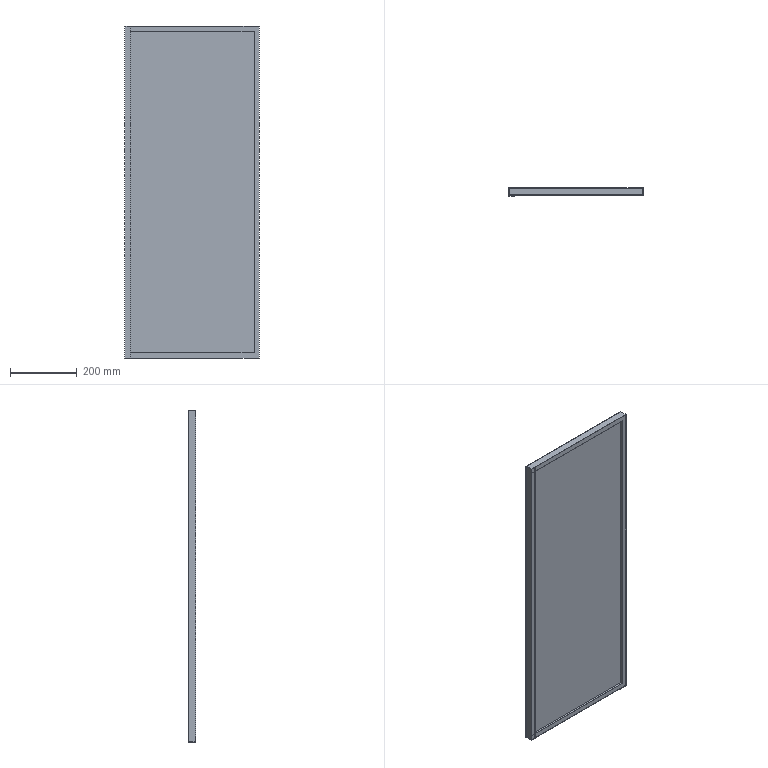Part | SolidWorks | features BossThin 2, ExtruThin 1 | 2 solids | 22 faces | box 401 x 23 x 992 mm | volume 497496 mm3 | plane 22
STEP:
#1=CARTESIAN_POINT('',(185.,-22.96,480.));
#2=VERTEX_POINT('',#1);
#3=CARTESIAN_POINT('',(-200.,-22.96,480.));
#4=VERTEX_POINT('',#3);
#5=CARTESIAN_POINT('',(200.,-22.96,480.));
#6=DIRECTION('',(-1.,0.,0.));
#7=VECTOR('',#6,1000.);
#8=LINE('',#5,#7);
#9=EDGE_CURVE('',#2,#4,#8,.T.);
#10=ORIENTED_EDGE('',*,*,#9,.F.);
#11=CARTESIAN_POINT('',(185.,-23.96,480.));
#12=VERTEX_POINT('',#11);
#13=CARTESIAN_POINT('',(185.,-22.96,480.));
#14=DIRECTION('',(0.,-1.,0.));
#15=VECTOR('',#14,1000.);
#16=LINE('',#13,#15);
#17=EDGE_CURVE('',#2,#12,#16,.T.);
#18=ORIENTED_EDGE('',*,*,#17,.T.);
#19=CARTESIAN_POINT('',(-200.,-23.96,480.));
#20=VERTEX_POINT('',#19);
#21=CARTESIAN_POINT('',(200.,-23.96,480.));
#22=DIRECTION('',(-1.,0.,0.));
#23=VECTOR('',#22,1000.);
#24=LINE('',#21,#23);
#25=EDGE_CURVE('',#12,#20,#24,.T.);
#26=ORIENTED_EDGE('',*,*,#25,.T.);
#27=CARTESIAN_POINT('',(-200.,-22.96,480.));
#28=DIRECTION('',(0.,-1.,0.));
#29=VECTOR('',#28,1000.);
#30=LINE('',#27,#29);
#31=EDGE_CURVE('',#4,#20,#30,.T.);
#32=ORIENTED_EDGE('',*,*,#31,.F.);
#33=EDGE_LOOP('',(#10,#18,#26,#32));
#34=FACE_OUTER_BOUND('',#33,.T.);
#35=CARTESIAN_POINT('',(200.,-22.96,480.));
#36=DIRECTION('',(0.,0.,-1.));
#37=DIRECTION('',(-1.,0.,0.));
#38=AXIS2_PLACEMENT_3D('',#35,#36,#37);
#39=PLANE('',#38);
#40=ADVANCED_FACE('',(#34),#39,.T.);
#41=CARTESIAN_POINT('',(185.,-23.96,-480.));
#42=VERTEX_POINT('',#41);
#43=CARTESIAN_POINT('',(-200.,-23.96,-480.));
#44=VERTEX_POINT('',#43);
#45=CARTESIAN_POINT('',(200.,-23.96,-480.));
#46=DIRECTION('',(-1.,0.,0.));
#47=VECTOR('',#46,1000.);
#48=LINE('',#45,#47);
#49=EDGE_CURVE('',#42,#44,#48,.T.);
#50=ORIENTED_EDGE('',*,*,#49,.F.);
#51=CARTESIAN_POINT('',(185.,-22.96,-480.));
#52=VERTEX_POINT('',#51);
#53=CARTESIAN_POINT('',(185.,-23.96,-480.));
#54=DIRECTION('',(0.,1.,0.));
#55=VECTOR('',#54,1000.);
#56=LINE('',#53,#55);
#57=EDGE_CURVE('',#42,#52,#56,.T.);
#58=ORIENTED_EDGE('',*,*,#57,.T.);
#59=CARTESIAN_POINT('',(-200.,-22.96,-480.));
#60=VERTEX_POINT('',#59);
#61=CARTESIAN_POINT('',(200.,-22.96,-480.));
#62=DIRECTION('',(-1.,0.,0.));
#63=VECTOR('',#62,1000.);
#64=LINE('',#61,#63);
#65=EDGE_CURVE('',#52,#60,#64,.T.);
#66=ORIENTED_EDGE('',*,*,#65,.T.);
#67=CARTESIAN_POINT('',(-200.,-23.96,-480.));
#68=DIRECTION('',(0.,1.,0.));
#69=VECTOR('',#68,1000.);
#70=LINE('',#67,#69);
#71=EDGE_CURVE('',#44,#60,#70,.T.);
#72=ORIENTED_EDGE('',*,*,#71,.F.);
#73=EDGE_LOOP('',(#50,#58,#66,#72));
#74=FACE_OUTER_BOUND('',#73,.T.);
#75=CARTESIAN_POINT('',(200.,-23.96,-480.));
#76=DIRECTION('',(0.,0.,1.));
#77=DIRECTION('',(1.,0.,0.));
#78=AXIS2_PLACEMENT_3D('',#75,#76,#77);
#79=PLANE('',#78);
#80=ADVANCED_FACE('',(#74),#79,.T.);
#81=CARTESIAN_POINT('',(199.,-22.96,495.));
#82=VERTEX_POINT('',#81);
#83=CARTESIAN_POINT('',(199.,-2.96,495.));
#84=VERTEX_POINT('',#83);
#85=CARTESIAN_POINT('',(199.,-2.96,495.));
#86=DIRECTION('',(0.,1.,0.));
#87=VECTOR('',#86,1000.);
#88=LINE('',#85,#87);
#89=EDGE_CURVE('',#82,#84,#88,.T.);
#90=ORIENTED_EDGE('',*,*,#89,.F.);
#91=CARTESIAN_POINT('',(-200.,-22.96,495.));
#92=VERTEX_POINT('',#91);
#93=CARTESIAN_POINT('',(200.,-22.96,495.));
#94=DIRECTION('',(-1.,0.,0.));
#95=VECTOR('',#94,1000.);
#96=LINE('',#93,#95);
#97=EDGE_CURVE('',#82,#92,#96,.T.);
#98=ORIENTED_EDGE('',*,*,#97,.T.);
#99=CARTESIAN_POINT('',(-200.,-2.96,495.));
#100=VERTEX_POINT('',#99);
#101=CARTESIAN_POINT('',(-200.,-2.96,495.));
#102=DIRECTION('',(0.,-1.,0.));
#103=VECTOR('',#102,1000.);
#104=LINE('',#101,#103);
#105=EDGE_CURVE('',#100,#92,#104,.T.);
#106=ORIENTED_EDGE('',*,*,#105,.F.);
#107=CARTESIAN_POINT('',(200.,-2.96,495.));
#108=DIRECTION('',(-1.,0.,0.));
#109=VECTOR('',#108,1000.);
#110=LINE('',#107,#109);
#111=EDGE_CURVE('',#84,#100,#110,.T.);
#112=ORIENTED_EDGE('',*,*,#111,.F.);
#113=EDGE_LOOP('',(#90,#98,#106,#112));
#114=FACE_OUTER_BOUND('',#113,.T.);
#115=CARTESIAN_POINT('',(200.,-2.96,495.));
#116=DIRECTION('',(0.,0.,-1.));
#117=DIRECTION('',(-1.,0.,0.));
#118=AXIS2_PLACEMENT_3D('',#115,#116,#117);
#119=PLANE('',#118);
#120=ADVANCED_FACE('',(#114),#119,.T.);
#121=CARTESIAN_POINT('',(199.,-2.96,-495.));
#122=VERTEX_POINT('',#121);
#123=CARTESIAN_POINT('',(199.,-2.96,-495.));
#124=DIRECTION('',(0.,0.,-1.));
#125=VECTOR('',#124,1000.);
#126=LINE('',#123,#125);
#127=EDGE_CURVE('',#84,#122,#126,.T.);
#128=ORIENTED_EDGE('',*,*,#127,.F.);
#129=ORIENTED_EDGE('',*,*,#111,.T.);
#130=CARTESIAN_POINT('',(-200.,-2.96,-495.));
#131=VERTEX_POINT('',#130);
#132=CARTESIAN_POINT('',(-200.,-2.96,-495.));
#133=DIRECTION('',(0.,0.,1.));
#134=VECTOR('',#133,1000.);
#135=LINE('',#132,#134);
#136=EDGE_CURVE('',#131,#100,#135,.T.);
#137=ORIENTED_EDGE('',*,*,#136,.F.);
#138=CARTESIAN_POINT('',(200.,-2.96,-495.));
#139=DIRECTION('',(-1.,0.,0.));
#140=VECTOR('',#139,1000.);
#141=LINE('',#138,#140);
#142=EDGE_CURVE('',#122,#131,#141,.T.);
#143=ORIENTED_EDGE('',*,*,#142,.F.);
#144=EDGE_LOOP('',(#128,#129,#137,#143));
#145=FACE_OUTER_BOUND('',#144,.T.);
#146=CARTESIAN_POINT('',(200.,-2.96,-495.));
#147=DIRECTION('',(0.,-1.,0.));
#148=DIRECTION('',(0.,0.,-1.));
#149=AXIS2_PLACEMENT_3D('',#146,#147,#148);
#150=PLANE('',#149);
#151=ADVANCED_FACE('',(#145),#150,.T.);
#152=CARTESIAN_POINT('',(199.,-22.96,-495.));
#153=VERTEX_POINT('',#152);
#154=CARTESIAN_POINT('',(199.,-2.96,-495.));
#155=DIRECTION('',(0.,-1.,0.));
#156=VECTOR('',#155,1000.);
#157=LINE('',#154,#156);
#158=EDGE_CURVE('',#122,#153,#157,.T.);
#159=ORIENTED_EDGE('',*,*,#158,.F.);
#160=ORIENTED_EDGE('',*,*,#142,.T.);
#161=CARTESIAN_POINT('',(-200.,-22.96,-495.));
#162=VERTEX_POINT('',#161);
#163=CARTESIAN_POINT('',(-200.,-2.96,-495.));
#164=DIRECTION('',(0.,1.,0.));
#165=VECTOR('',#164,1000.);
#166=LINE('',#163,#165);
#167=EDGE_CURVE('',#162,#131,#166,.T.);
#168=ORIENTED_EDGE('',*,*,#167,.F.);
#169=CARTESIAN_POINT('',(200.,-22.96,-495.));
#170=DIRECTION('',(-1.,0.,0.));
#171=VECTOR('',#170,1000.);
#172=LINE('',#169,#171);
#173=EDGE_CURVE('',#153,#162,#172,.T.);
#174=ORIENTED_EDGE('',*,*,#173,.F.);
#175=EDGE_LOOP('',(#159,#160,#168,#174));
#176=FACE_OUTER_BOUND('',#175,.T.);
#177=CARTESIAN_POINT('',(200.,-2.96,-495.));
#178=DIRECTION('',(0.,0.,1.));
#179=DIRECTION('',(1.,0.,0.));
#180=AXIS2_PLACEMENT_3D('',#177,#178,#179);
#181=PLANE('',#180);
#182=ADVANCED_FACE('',(#176),#181,.T.);
#183=CARTESIAN_POINT('',(199.,-22.96,-496.));
#184=DIRECTION('',(0.,0.,1.));
#185=VECTOR('',#184,1000.);
#186=LINE('',#183,#185);
#187=EDGE_CURVE('',#153,#82,#186,.T.);
#188=ORIENTED_EDGE('',*,*,#187,.F.);
#189=ORIENTED_EDGE('',*,*,#173,.T.);
#190=CARTESIAN_POINT('',(-200.,-22.96,-495.));
#191=DIRECTION('',(0.,0.,-1.));
#192=VECTOR('',#191,1000.);
#193=LINE('',#190,#192);
#194=EDGE_CURVE('',#60,#162,#193,.T.);
#195=ORIENTED_EDGE('',*,*,#194,.F.);
#196=ORIENTED_EDGE('',*,*,#65,.F.);
#197=CARTESIAN_POINT('',(185.,-22.96,-496.));
#198=DIRECTION('',(0.,0.,1.));
#199=VECTOR('',#198,1000.);
#200=LINE('',#197,#199);
#201=EDGE_CURVE('',#52,#2,#200,.T.);
#202=ORIENTED_EDGE('',*,*,#201,.T.);
#203=ORIENTED_EDGE('',*,*,#9,.T.);
#204=CARTESIAN_POINT('',(-200.,-22.96,495.));
#205=DIRECTION('',(0.,0.,-1.));
#206=VECTOR('',#205,1000.);
#207=LINE('',#204,#206);
#208=EDGE_CURVE('',#92,#4,#207,.T.);
#209=ORIENTED_EDGE('',*,*,#208,.F.);
#210=ORIENTED_EDGE('',*,*,#97,.F.);
#211=EDGE_LOOP('',(#188,#189,#195,#196,#202,#203,#209,#210));
#212=FACE_OUTER_BOUND('',#211,.T.);
#213=CARTESIAN_POINT('',(200.,-22.96,-495.));
#214=DIRECTION('',(0.,1.,0.));
#215=DIRECTION('',(0.,0.,1.));
#216=AXIS2_PLACEMENT_3D('',#213,#214,#215);
#217=PLANE('',#216);
#218=ADVANCED_FACE('',(#212),#217,.T.);
#219=CARTESIAN_POINT('',(200.,-23.96,-496.));
#220=VERTEX_POINT('',#219);
#221=CARTESIAN_POINT('',(-200.,-23.96,-496.));
#222=VERTEX_POINT('',#221);
#223=CARTESIAN_POINT('',(200.,-23.96,-496.));
#224=DIRECTION('',(-1.,0.,0.));
#225=VECTOR('',#224,1000.);
#226=LINE('',#223,#225);
#227=EDGE_CURVE('',#220,#222,#226,.T.);
#228=ORIENTED_EDGE('',*,*,#227,.F.);
#229=CARTESIAN_POINT('',(200.,-23.96,496.));
#230=VERTEX_POINT('',#229);
#231=CARTESIAN_POINT('',(200.,-23.96,495.));
#232=DIRECTION('',(0.,0.,-1.));
#233=VECTOR('',#232,1000.);
#234=LINE('',#231,#233);
#235=EDGE_CURVE('',#230,#220,#234,.T.);
#236=ORIENTED_EDGE('',*,*,#235,.F.);
#237=CARTESIAN_POINT('',(-200.,-23.96,496.));
#238=VERTEX_POINT('',#237);
#239=CARTESIAN_POINT('',(200.,-23.96,496.));
#240=DIRECTION('',(-1.,0.,0.));
#241=VECTOR('',#240,1000.);
#242=LINE('',#239,#241);
#243=EDGE_CURVE('',#230,#238,#242,.T.);
#244=ORIENTED_EDGE('',*,*,#243,.T.);
#245=CARTESIAN_POINT('',(-200.,-23.96,495.));
#246=DIRECTION('',(0.,0.,-1.));
#247=VECTOR('',#246,1000.);
#248=LINE('',#245,#247);
#249=EDGE_CURVE('',#238,#20,#248,.T.);
#250=ORIENTED_EDGE('',*,*,#249,.T.);
#251=ORIENTED_EDGE('',*,*,#25,.F.);
#252=CARTESIAN_POINT('',(185.,-23.96,-496.));
#253=DIRECTION('',(0.,0.,1.));
#254=VECTOR('',#253,1000.);
#255=LINE('',#252,#254);
#256=EDGE_CURVE('',#42,#12,#255,.T.);
#257=ORIENTED_EDGE('',*,*,#256,.F.);
#258=ORIENTED_EDGE('',*,*,#49,.T.);
#259=CARTESIAN_POINT('',(-200.,-23.96,-495.));
#260=DIRECTION('',(0.,0.,-1.));
#261=VECTOR('',#260,1000.);
#262=LINE('',#259,#261);
#263=EDGE_CURVE('',#44,#222,#262,.T.);
#264=ORIENTED_EDGE('',*,*,#263,.T.);
#265=EDGE_LOOP('',(#228,#236,#244,#250,#251,#257,#258,#264));
#266=FACE_OUTER_BOUND('',#265,.T.);
#267=CARTESIAN_POINT('',(200.,-23.96,-495.));
#268=DIRECTION('',(0.,1.,0.));
#269=DIRECTION('',(0.,0.,1.));
#270=AXIS2_PLACEMENT_3D('',#267,#268,#269);
#271=PLANE('',#270);
#272=ADVANCED_FACE('',(#266),#271,.F.);
#273=CARTESIAN_POINT('',(-200.,-1.96,-496.));
#274=VERTEX_POINT('',#273);
#275=CARTESIAN_POINT('',(-200.,-2.96,-496.));
#276=DIRECTION('',(0.,1.,0.));
#277=VECTOR('',#276,1000.);
#278=LINE('',#275,#277);
#279=EDGE_CURVE('',#222,#274,#278,.T.);
#280=ORIENTED_EDGE('',*,*,#279,.T.);
#281=CARTESIAN_POINT('',(200.,-1.96,-496.));
#282=VERTEX_POINT('',#281);
#283=CARTESIAN_POINT('',(200.,-1.96,-496.));
#284=DIRECTION('',(-1.,0.,0.));
#285=VECTOR('',#284,1000.);
#286=LINE('',#283,#285);
#287=EDGE_CURVE('',#282,#274,#286,.T.);
#288=ORIENTED_EDGE('',*,*,#287,.F.);
#289=CARTESIAN_POINT('',(200.,-2.96,-496.));
#290=DIRECTION('',(0.,1.,0.));
#291=VECTOR('',#290,1000.);
#292=LINE('',#289,#291);
#293=EDGE_CURVE('',#220,#282,#292,.T.);
#294=ORIENTED_EDGE('',*,*,#293,.F.);
#295=ORIENTED_EDGE('',*,*,#227,.T.);
#296=EDGE_LOOP('',(#280,#288,#294,#295));
#297=FACE_OUTER_BOUND('',#296,.T.);
#298=CARTESIAN_POINT('',(200.,-2.96,-496.));
#299=DIRECTION('',(0.,0.,1.));
#300=DIRECTION('',(1.,0.,0.));
#301=AXIS2_PLACEMENT_3D('',#298,#299,#300);
#302=PLANE('',#301);
#303=ADVANCED_FACE('',(#297),#302,.F.);
#304=CARTESIAN_POINT('',(-200.,-1.96,496.));
#305=VERTEX_POINT('',#304);
#306=CARTESIAN_POINT('',(-200.,-1.96,-495.));
#307=DIRECTION('',(0.,0.,1.));
#308=VECTOR('',#307,1000.);
#309=LINE('',#306,#308);
#310=EDGE_CURVE('',#274,#305,#309,.T.);
#311=ORIENTED_EDGE('',*,*,#310,.T.);
#312=CARTESIAN_POINT('',(200.,-1.96,496.));
#313=VERTEX_POINT('',#312);
#314=CARTESIAN_POINT('',(200.,-1.96,496.));
#315=DIRECTION('',(-1.,0.,0.));
#316=VECTOR('',#315,1000.);
#317=LINE('',#314,#316);
#318=EDGE_CURVE('',#313,#305,#317,.T.);
#319=ORIENTED_EDGE('',*,*,#318,.F.);
#320=CARTESIAN_POINT('',(200.,-1.96,-495.));
#321=DIRECTION('',(0.,0.,1.));
#322=VECTOR('',#321,1000.);
#323=LINE('',#320,#322);
#324=EDGE_CURVE('',#282,#313,#323,.T.);
#325=ORIENTED_EDGE('',*,*,#324,.F.);
#326=ORIENTED_EDGE('',*,*,#287,.T.);
#327=EDGE_LOOP('',(#311,#319,#325,#326));
#328=FACE_OUTER_BOUND('',#327,.T.);
#329=CARTESIAN_POINT('',(200.,-1.96,-495.));
#330=DIRECTION('',(0.,-1.,0.));
#331=DIRECTION('',(0.,0.,-1.));
#332=AXIS2_PLACEMENT_3D('',#329,#330,#331);
#333=PLANE('',#332);
#334=ADVANCED_FACE('',(#328),#333,.F.);
#335=ORIENTED_EDGE('',*,*,#318,.T.);
#336=CARTESIAN_POINT('',(-200.,-2.96,496.));
#337=DIRECTION('',(0.,-1.,0.));
#338=VECTOR('',#337,1000.);
#339=LINE('',#336,#338);
#340=EDGE_CURVE('',#305,#238,#339,.T.);
#341=ORIENTED_EDGE('',*,*,#340,.T.);
#342=ORIENTED_EDGE('',*,*,#243,.F.);
#343=CARTESIAN_POINT('',(200.,-2.96,496.));
#344=DIRECTION('',(0.,-1.,0.));
#345=VECTOR('',#344,1000.);
#346=LINE('',#343,#345);
#347=EDGE_CURVE('',#313,#230,#346,.T.);
#348=ORIENTED_EDGE('',*,*,#347,.F.);
#349=EDGE_LOOP('',(#335,#341,#342,#348));
#350=FACE_OUTER_BOUND('',#349,.T.);
#351=CARTESIAN_POINT('',(200.,-2.96,496.));
#352=DIRECTION('',(0.,0.,-1.));
#353=DIRECTION('',(-1.,0.,0.));
#354=AXIS2_PLACEMENT_3D('',#351,#352,#353);
#355=PLANE('',#354);
#356=ADVANCED_FACE('',(#350),#355,.F.);
#357=ORIENTED_EDGE('',*,*,#235,.T.);
#358=ORIENTED_EDGE('',*,*,#293,.T.);
#359=ORIENTED_EDGE('',*,*,#324,.T.);
#360=ORIENTED_EDGE('',*,*,#347,.T.);
#361=EDGE_LOOP('',(#357,#358,#359,#360));
#362=FACE_OUTER_BOUND('',#361,.T.);
#363=CARTESIAN_POINT('',(200.,-23.96,480.));
#364=DIRECTION('',(-1.,0.,0.));
#365=DIRECTION('',(0.,0.,1.));
#366=AXIS2_PLACEMENT_3D('',#363,#364,#365);
#367=PLANE('',#366);
#368=ADVANCED_FACE('',(#362),#367,.F.);
#369=ORIENTED_EDGE('',*,*,#249,.F.);
#370=ORIENTED_EDGE('',*,*,#340,.F.);
#371=ORIENTED_EDGE('',*,*,#310,.F.);
#372=ORIENTED_EDGE('',*,*,#279,.F.);
#373=ORIENTED_EDGE('',*,*,#263,.F.);
#374=ORIENTED_EDGE('',*,*,#71,.T.);
#375=ORIENTED_EDGE('',*,*,#194,.T.);
#376=ORIENTED_EDGE('',*,*,#167,.T.);
#377=ORIENTED_EDGE('',*,*,#136,.T.);
#378=ORIENTED_EDGE('',*,*,#105,.T.);
#379=ORIENTED_EDGE('',*,*,#208,.T.);
#380=ORIENTED_EDGE('',*,*,#31,.T.);
#381=EDGE_LOOP('',(#369,#370,#371,#372,#373,#374,#375,#376,#377,#378,#379,#380));
#382=FACE_OUTER_BOUND('',#381,.T.);
#383=CARTESIAN_POINT('',(-200.,-23.96,480.));
#384=DIRECTION('',(-1.,0.,0.));
#385=DIRECTION('',(0.,0.,1.));
#386=AXIS2_PLACEMENT_3D('',#383,#384,#385);
#387=PLANE('',#386);
#388=ADVANCED_FACE('',(#382),#387,.T.);
#389=ORIENTED_EDGE('',*,*,#187,.T.);
#390=ORIENTED_EDGE('',*,*,#89,.T.);
#391=ORIENTED_EDGE('',*,*,#127,.T.);
#392=ORIENTED_EDGE('',*,*,#158,.T.);
#393=EDGE_LOOP('',(#389,#390,#391,#392));
#394=FACE_OUTER_BOUND('',#393,.T.);
#395=CARTESIAN_POINT('',(199.,-1.96,-496.));
#396=DIRECTION('',(-1.,0.,0.));
#397=DIRECTION('',(0.,0.,1.));
#398=AXIS2_PLACEMENT_3D('',#395,#396,#397);
#399=PLANE('',#398);
#400=ADVANCED_FACE('',(#394),#399,.T.);
#401=ORIENTED_EDGE('',*,*,#17,.F.);
#402=ORIENTED_EDGE('',*,*,#201,.F.);
#403=ORIENTED_EDGE('',*,*,#57,.F.);
#404=ORIENTED_EDGE('',*,*,#256,.T.);
#405=EDGE_LOOP('',(#401,#402,#403,#404));
#406=FACE_OUTER_BOUND('',#405,.T.);
#407=CARTESIAN_POINT('',(185.,-23.96,-496.));
#408=DIRECTION('',(1.,0.,0.));
#409=DIRECTION('',(0.,0.,-1.));
#410=AXIS2_PLACEMENT_3D('',#407,#408,#409);
#411=PLANE('',#410);
#412=ADVANCED_FACE('',(#406),#411,.F.);
#413=CLOSED_SHELL('',(#40,#80,#120,#151,#182,#218,#272,#303,#334,#356,#368,#388,#400,#412));
#414=MANIFOLD_SOLID_BREP('',#413);
#415=CARTESIAN_POINT('',(-201.,-24.96,496.));
#416=VERTEX_POINT('',#415);
#417=CARTESIAN_POINT('',(-185.,-24.96,496.));
#418=VERTEX_POINT('',#417);
#419=CARTESIAN_POINT('',(-200.,-24.96,496.));
#420=DIRECTION('',(1.,0.,0.));
#421=VECTOR('',#420,1000.);
#422=LINE('',#419,#421);
#423=EDGE_CURVE('',#416,#418,#422,.T.);
#424=ORIENTED_EDGE('',*,*,#423,.F.);
#425=CARTESIAN_POINT('',(-201.,-24.96,-496.));
#426=VERTEX_POINT('',#425);
#427=CARTESIAN_POINT('',(-201.,-24.96,-496.));
#428=DIRECTION('',(0.,0.,1.));
#429=VECTOR('',#428,1000.);
#430=LINE('',#427,#429);
#431=EDGE_CURVE('',#426,#416,#430,.T.);
#432=ORIENTED_EDGE('',*,*,#431,.F.);
#433=CARTESIAN_POINT('',(-185.,-24.96,-496.));
#434=VERTEX_POINT('',#433);
#435=CARTESIAN_POINT('',(-200.,-24.96,-496.));
#436=DIRECTION('',(1.,0.,0.));
#437=VECTOR('',#436,1000.);
#438=LINE('',#435,#437);
#439=EDGE_CURVE('',#426,#434,#438,.T.);
#440=ORIENTED_EDGE('',*,*,#439,.T.);
#441=CARTESIAN_POINT('',(-185.,-24.96,-496.));
#442=DIRECTION('',(0.,0.,1.));
#443=VECTOR('',#442,1000.);
#444=LINE('',#441,#443);
#445=EDGE_CURVE('',#434,#418,#444,.T.);
#446=ORIENTED_EDGE('',*,*,#445,.T.);
#447=EDGE_LOOP('',(#424,#432,#440,#446));
#448=FACE_OUTER_BOUND('',#447,.T.);
#449=CARTESIAN_POINT('',(-200.,-24.96,-496.));
#450=DIRECTION('',(0.,-1.,0.));
#451=DIRECTION('',(0.,0.,-1.));
#452=AXIS2_PLACEMENT_3D('',#449,#450,#451);
#453=PLANE('',#452);
#454=ADVANCED_FACE('',(#448),#453,.T.);
#455=CARTESIAN_POINT('',(-201.,-1.96,496.));
#456=VERTEX_POINT('',#455);
#457=CARTESIAN_POINT('',(-201.,-1.96,496.));
#458=DIRECTION('',(0.,-1.,0.));
#459=VECTOR('',#458,1000.);
#460=LINE('',#457,#459);
#461=EDGE_CURVE('',#456,#416,#460,.T.);
#462=ORIENTED_EDGE('',*,*,#461,.F.);
#463=CARTESIAN_POINT('',(-201.,-1.96,-496.));
#464=VERTEX_POINT('',#463);
#465=CARTESIAN_POINT('',(-201.,-1.96,-496.));
#466=DIRECTION('',(0.,0.,1.));
#467=VECTOR('',#466,1000.);
#468=LINE('',#465,#467);
#469=EDGE_CURVE('',#464,#456,#468,.T.);
#470=ORIENTED_EDGE('',*,*,#469,.F.);
#471=CARTESIAN_POINT('',(-201.,-1.96,-496.));
#472=DIRECTION('',(0.,-1.,0.));
#473=VECTOR('',#472,1000.);
#474=LINE('',#471,#473);
#475=EDGE_CURVE('',#464,#426,#474,.T.);
#476=ORIENTED_EDGE('',*,*,#475,.T.);
#477=ORIENTED_EDGE('',*,*,#431,.T.);
#478=EDGE_LOOP('',(#462,#470,#476,#477));
#479=FACE_OUTER_BOUND('',#478,.T.);
#480=CARTESIAN_POINT('',(-201.,-1.96,-496.));
#481=DIRECTION('',(-1.,0.,0.));
#482=DIRECTION('',(0.,0.,1.));
#483=AXIS2_PLACEMENT_3D('',#480,#481,#482);
#484=PLANE('',#483);
#485=ADVANCED_FACE('',(#479),#484,.T.);
#486=CARTESIAN_POINT('',(-200.,-1.96,496.));
#487=VERTEX_POINT('',#486);
#488=CARTESIAN_POINT('',(-201.,-1.96,496.));
#489=DIRECTION('',(1.,0.,0.));
#490=VECTOR('',#489,1000.);
#491=LINE('',#488,#490);
#492=EDGE_CURVE('',#456,#487,#491,.T.);
#493=ORIENTED_EDGE('',*,*,#492,.T.);
#494=CARTESIAN_POINT('',(-200.,-1.96,-496.));
#495=VERTEX_POINT('',#494);
#496=CARTESIAN_POINT('',(-200.,-1.96,-496.));
#497=DIRECTION('',(0.,0.,1.));
#498=VECTOR('',#497,1000.);
#499=LINE('',#496,#498);
#500=EDGE_CURVE('',#495,#487,#499,.T.);
#501=ORIENTED_EDGE('',*,*,#500,.F.);
#502=CARTESIAN_POINT('',(-201.,-1.96,-496.));
#503=DIRECTION('',(1.,0.,0.));
#504=VECTOR('',#503,1000.);
#505=LINE('',#502,#504);
#506=EDGE_CURVE('',#464,#495,#505,.T.);
#507=ORIENTED_EDGE('',*,*,#506,.F.);
#508=ORIENTED_EDGE('',*,*,#469,.T.);
#509=EDGE_LOOP('',(#493,#501,#507,#508));
#510=FACE_OUTER_BOUND('',#509,.T.);
#511=CARTESIAN_POINT('',(-201.,-1.96,-496.));
#512=DIRECTION('',(0.,-1.,0.));
#513=DIRECTION('',(0.,0.,-1.));
#514=AXIS2_PLACEMENT_3D('',#511,#512,#513);
#515=PLANE('',#514);
#516=ADVANCED_FACE('',(#510),#515,.F.);
#517=CARTESIAN_POINT('',(-200.,-23.96,496.));
#518=VERTEX_POINT('',#517);
#519=CARTESIAN_POINT('',(-200.,-1.96,496.));
#520=DIRECTION('',(0.,-1.,0.));
#521=VECTOR('',#520,1000.);
#522=LINE('',#519,#521);
#523=EDGE_CURVE('',#487,#518,#522,.T.);
#524=ORIENTED_EDGE('',*,*,#523,.T.);
#525=CARTESIAN_POINT('',(-200.,-23.96,-496.));
#526=VERTEX_POINT('',#525);
#527=CARTESIAN_POINT('',(-200.,-23.96,-496.));
#528=DIRECTION('',(0.,0.,1.));
#529=VECTOR('',#528,1000.);
#530=LINE('',#527,#529);
#531=EDGE_CURVE('',#526,#518,#530,.T.);
#532=ORIENTED_EDGE('',*,*,#531,.F.);
#533=CARTESIAN_POINT('',(-200.,-1.96,-496.));
#534=DIRECTION('',(0.,-1.,0.));
#535=VECTOR('',#534,1000.);
#536=LINE('',#533,#535);
#537=EDGE_CURVE('',#495,#526,#536,.T.);
#538=ORIENTED_EDGE('',*,*,#537,.F.);
#539=ORIENTED_EDGE('',*,*,#500,.T.);
#540=EDGE_LOOP('',(#524,#532,#538,#539));
#541=FACE_OUTER_BOUND('',#540,.T.);
#542=CARTESIAN_POINT('',(-200.,-1.96,-496.));
#543=DIRECTION('',(-1.,0.,0.));
#544=DIRECTION('',(0.,0.,1.));
#545=AXIS2_PLACEMENT_3D('',#542,#543,#544);
#546=PLANE('',#545);
#547=ADVANCED_FACE('',(#541),#546,.F.);
#548=CARTESIAN_POINT('',(-185.,-23.96,496.));
#549=VERTEX_POINT('',#548);
#550=CARTESIAN_POINT('',(-200.,-23.96,496.));
#551=DIRECTION('',(1.,0.,0.));
#552=VECTOR('',#551,1000.);
#553=LINE('',#550,#552);
#554=EDGE_CURVE('',#518,#549,#553,.T.);
#555=ORIENTED_EDGE('',*,*,#554,.T.);
#556=CARTESIAN_POINT('',(-185.,-23.96,-496.));
#557=VERTEX_POINT('',#556);
#558=CARTESIAN_POINT('',(-185.,-23.96,-496.));
#559=DIRECTION('',(0.,0.,1.));
#560=VECTOR('',#559,1000.);
#561=LINE('',#558,#560);
#562=EDGE_CURVE('',#557,#549,#561,.T.);
#563=ORIENTED_EDGE('',*,*,#562,.F.);
#564=CARTESIAN_POINT('',(-200.,-23.96,-496.));
#565=DIRECTION('',(1.,0.,0.));
#566=VECTOR('',#565,1000.);
#567=LINE('',#564,#566);
#568=EDGE_CURVE('',#526,#557,#567,.T.);
#569=ORIENTED_EDGE('',*,*,#568,.F.);
#570=ORIENTED_EDGE('',*,*,#531,.T.);
#571=EDGE_LOOP('',(#555,#563,#569,#570));
#572=FACE_OUTER_BOUND('',#571,.T.);
#573=CARTESIAN_POINT('',(-200.,-23.96,-496.));
#574=DIRECTION('',(0.,-1.,0.));
#575=DIRECTION('',(0.,0.,-1.));
#576=AXIS2_PLACEMENT_3D('',#573,#574,#575);
#577=PLANE('',#576);
#578=ADVANCED_FACE('',(#572),#577,.F.);
#579=CARTESIAN_POINT('',(-185.,-23.96,496.));
#580=DIRECTION('',(0.,-1.,0.));
#581=VECTOR('',#580,1000.);
#582=LINE('',#579,#581);
#583=EDGE_CURVE('',#549,#418,#582,.T.);
#584=ORIENTED_EDGE('',*,*,#583,.T.);
#585=ORIENTED_EDGE('',*,*,#445,.F.);
#586=CARTESIAN_POINT('',(-185.,-23.96,-496.));
#587=DIRECTION('',(0.,-1.,0.));
#588=VECTOR('',#587,1000.);
#589=LINE('',#586,#588);
#590=EDGE_CURVE('',#557,#434,#589,.T.);
#591=ORIENTED_EDGE('',*,*,#590,.F.);
#592=ORIENTED_EDGE('',*,*,#562,.T.);
#593=EDGE_LOOP('',(#584,#585,#591,#592));
#594=FACE_OUTER_BOUND('',#593,.T.);
#595=CARTESIAN_POINT('',(-185.,-23.96,-496.));
#596=DIRECTION('',(-1.,0.,0.));
#597=DIRECTION('',(0.,0.,1.));
#598=AXIS2_PLACEMENT_3D('',#595,#596,#597);
#599=PLANE('',#598);
#600=ADVANCED_FACE('',(#594),#599,.F.);
#601=ORIENTED_EDGE('',*,*,#439,.F.);
#602=ORIENTED_EDGE('',*,*,#475,.F.);
#603=ORIENTED_EDGE('',*,*,#506,.T.);
#604=ORIENTED_EDGE('',*,*,#537,.T.);
#605=ORIENTED_EDGE('',*,*,#568,.T.);
#606=ORIENTED_EDGE('',*,*,#590,.T.);
#607=EDGE_LOOP('',(#601,#602,#603,#604,#605,#606));
#608=FACE_OUTER_BOUND('',#607,.T.);
#609=CARTESIAN_POINT('',(-185.,-24.96,-496.));
#610=DIRECTION('',(0.,0.,-1.));
#611=DIRECTION('',(-1.,0.,0.));
#612=AXIS2_PLACEMENT_3D('',#609,#610,#611);
#613=PLANE('',#612);
#614=ADVANCED_FACE('',(#608),#613,.T.);
#615=ORIENTED_EDGE('',*,*,#423,.T.);
#616=ORIENTED_EDGE('',*,*,#583,.F.);
#617=ORIENTED_EDGE('',*,*,#554,.F.);
#618=ORIENTED_EDGE('',*,*,#523,.F.);
#619=ORIENTED_EDGE('',*,*,#492,.F.);
#620=ORIENTED_EDGE('',*,*,#461,.T.);
#621=EDGE_LOOP('',(#615,#616,#617,#618,#619,#620));
#622=FACE_OUTER_BOUND('',#621,.T.);
#623=CARTESIAN_POINT('',(-185.,-24.96,496.));
#624=DIRECTION('',(0.,0.,-1.));
#625=DIRECTION('',(-1.,0.,0.));
#626=AXIS2_PLACEMENT_3D('',#623,#624,#625);
#627=PLANE('',#626);
#628=ADVANCED_FACE('',(#622),#627,.F.);
#629=CLOSED_SHELL('',(#454,#485,#516,#547,#578,#600,#614,#628));
#630=MANIFOLD_SOLID_BREP('',#629);
#631=CARTESIAN_POINT('',(0.,0.,0.));
#632=DIRECTION('',(0.,0.,1.));
#633=DIRECTION('',(1.,0.,0.));
#634=AXIS2_PLACEMENT_3D('',#631,#632,#633);
#635=(LENGTH_UNIT()NAMED_UNIT(*)SI_UNIT(.MILLI.,.METRE.));
#636=UNCERTAINTY_MEASURE_WITH_UNIT(LENGTH_MEASURE(0.00001),#635,'','');
#637=(NAMED_UNIT(*)PLANE_ANGLE_UNIT()SI_UNIT($,.RADIAN.));
#638=(NAMED_UNIT(*)SI_UNIT($,.STERADIAN.)SOLID_ANGLE_UNIT());
#639=(GEOMETRIC_REPRESENTATION_CONTEXT(3)GLOBAL_UNCERTAINTY_ASSIGNED_CONTEXT((#636))GLOBAL_UNIT_ASSIGNED_CONTEXT((#635,#637,#638))REPRESENTATION_CONTEXT('',''));
#640=ADVANCED_BREP_SHAPE_REPRESENTATION('',(#414,#630,#634),#639);